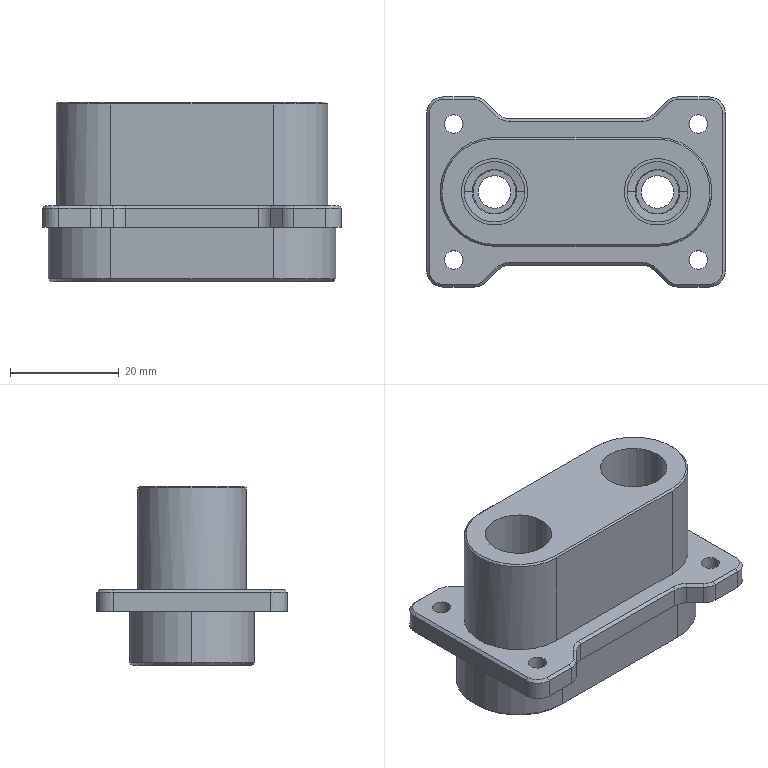NC program | NX | posted with a generic post | part box 55 x 35 x 33 mm
Whole program:
N10 G17 G21 G94 G90
(PLANAR_MILL , TOOL : D50面刀)
N12 T01 M6
N14 G54
N16 G17 G0 G90 X59.5 Y0. S3500 M3
N18 G43 Z30. H1
N20 Z2.
N22 G94 G1 Z0. F800.
N24 X29.5
N26 X-29.5
N28 X-59.5
N30 Z2.
N32 G0 Z30.
N34 M5
(ADAPTIVE_MILLING , TOOL : D6开粗)
N36 T02 M6
N38 G54
N40 G17 G0 G90 X-37.082 Y-1.951 S5500 M3
N42 G43 Z30. H2
N44 Z-6.85
N46 G94 G1 X-36.933 Y-1.933 Z-7.787 F2500.
N48 X-36.784 Y-1.915 Z-8.158
N50 X-36.635 Y-1.896 Z-8.43
N52 X-36.486 Y-1.878 Z-8.65
N54 X-36.337 Y-1.859 Z-8.834
N56 X-36.188 Y-1.841 Z-8.992
N58 X-36.04 Y-1.823 Z-9.13
N60 X-35.891 Y-1.804 Z-9.25
N62 X-35.742 Y-1.786 Z-9.355
N64 X-35.593 Y-1.767 Z-9.448
N66 X-35.444 Y-1.749 Z-9.529
N68 X-35.295 Y-1.731 Z-9.6
N70 X-35.146 Y-1.712 Z-9.66
N72 X-34.997 Y-1.694 Z-9.712
N74 X-34.849 Y-1.675 Z-9.755
N76 X-34.7 Y-1.657 Z-9.789
N78 X-34.551 Y-1.639 Z-9.816
N80 X-34.402 Y-1.62 Z-9.835
N82 X-34.253 Y-1.602 Z-9.846
N84 X-34.104 Y-1.583 Z-9.85
N86 X-33.036 Y-1.451
N88 G3 X-32.602 Y-1.181 R0.61
N90 X-32.052 Y0.418 R3.749
N92 X-31.757 Y5.239 R34.791
N94 G1 X-31.719 Y18.308
N96 G2 X-30.257 Y20.605 R3.404
N98 X-27.007 Y21.854 R7.591
N100 X-21.623 Y22.205 R36.427
N102 G1 X-15.224 Y22.23
N104 X27.708 Y22.226
N106 G2 X30.104 Y20.755 R3.359
N108 X31.371 Y17.403 R7.706
N110 X31.707 Y11.819 R39.238
N112 G1 X31.729 Y4.819
N114 X31.727 Y-18.149
N116 G2 X30.405 Y-20.517 R3.217
N118 X27.196 Y-21.824 R7.156
N120 X22.015 Y-22.193 R33.325
N122 G1 X15.015 Y-22.223
N124 X-27.647 Y-22.228
N126 G2 X-30.017 Y-20.909 R3.219
N128 X-31.327 Y-17.701 R7.175
N130 X-31.694 Y-12.72 R32.061
N132 X-31.711 Y-3.192 R449.115
N134 X-31.242 Y0.643 R185.492
N136 G3 X-30.94 Y8.619 R86.106
N138 G1 X-30.917 Y16.308
N140 G2 X-28.825 Y19.681 R4.499
N142 X-24.992 Y21.042 R9.424
N144 X-19.008 Y21.406 R44.006
N146 G1 X-12.408 Y21.43
N148 X25.608 Y21.427
N150 G2 X29.121 Y19.407 R4.476
N152 X30.525 Y15.588 R9.179
N154 X30.902 Y9.705 R41.842
N156 G1 X30.929 Y2.605
N158 X30.926 Y-16.168
N160 G2 X28.878 Y-19.655 R4.431
N162 X25.248 Y-20.997 R9.046
N164 X19.667 Y-21.389 R38.056
N166 G1 X13.067 Y-21.423
N168 X-25.667 Y-21.426
N170 G2 X-29.158 Y-19.377 R4.444
N172 X-30.519 Y-15.65 R9.202
N174 X-30.9 Y-9.867 R40.724
N176 X-30.878 Y-3.868 R96.242
N178 G1 X-30.404 Y1.28
N180 G3 X-30.135 Y10.714 R133.466
N182 G2 X-30.095 Y14.907 R80.862
N184 X-27.424 Y18.917 R5.279
N186 X-23.263 Y20.254 R11.082
N188 X-16.577 Y20.611 R53.243
N190 G1 X-9.977 Y20.629
N192 X23.823 Y20.627
N194 G2 X28.316 Y18.084 R5.223
N196 X29.708 Y14.049 R10.439
N198 X30.103 Y7.666 R46.614
N200 G1 X30.129 Y3.266
N202 X30.128 Y-14.268
N204 G2 X27.533 Y-18.852 R5.225
N206 X23.385 Y-20.231 R10.759
N208 X17.301 Y-20.596 R47.863
N210 G1 X10.701 Y-20.623
N212 X-23.768 Y-20.628
N214 G2 X-28.404 Y-17.959 R5.26
N216 X-29.734 Y-13.897 R10.825
N218 X-30.098 Y-8.013 R46.197
N220 X-29.753 Y-0.507 R61.506
N222 G3 X-29.338 Y10.918 R136.638
N224 G2 X-29.245 Y13.909 R23.846
N226 X-26.349 Y18.035 R5.781
N228 X-22.095 Y19.413 R11.597
N230 X-15.512 Y19.803 R50.356
N232 G1 X-8.912 Y19.829
N234 X22.188 Y19.827
N236 G2 X26.329 Y18.348 R5.861
N238 X28.494 Y14.571 R8.022
N240 X29.2 Y9.531 R22.93
N242 X29.322 Y2.969 R160.009
N244 G1 X29.541 Y1.782
N246 X29.65 Y0.018
N248 G3 X29.383 Y-4.527 R166.198
N250 X29.319 Y-13.068 R660.599
N252 G2 X26.406 Y-18.003 R5.745
N254 X22.144 Y-19.401 R11.531
N256 X15.56 Y-19.796 R50.199
N258 G1 X8.56 Y-19.823
N260 X-22.267 Y-19.826
N262 G2 X-27.607 Y-16.734 R5.839
N264 X-28.933 Y-12.461 R11.993
N266 X-29.178 Y-3.571 R47.724
N268 G1 X-29.398 Y-2.708
N270 X-29.624 Y-0.88
N272 X-29.618 Y0.964
N274 X-29.381 Y2.792
N276 G3 X-28.648 Y7.519 R17.936
N278 G1 X-28.51 Y12.137
N280 G2 X-25.151 Y17.278 R6.243
N282 X-20.671 Y18.631 R12.837
N284 X-13.785 Y19.006 R56.828
N286 G1 X-7.186 Y19.029
N288 X20.614 Y19.028
N290 G2 X23.929 Y18.419 R7.485
N292 X27.126 Y14.947 R6.784
N294 X28.247 Y10.198 R15.536
N296 X28.489 Y5.706 R68.839
N298 X29.221 Y3.52 R19.948
N300 G1 X29.541 Y1.782
N302 X29.65 Y0.018
N304 X29.545 Y-1.75
N306 X29.228 Y-3.491
N308 G3 X28.662 Y-6.813 R11.878
N310 X28.515 Y-11.988 R178.125
N312 G2 X25.189 Y-17.254 R6.207
N314 X20.613 Y-18.633 R12.848
N316 X13.527 Y-19.003 R59.413
N318 G1 X6.827 Y-19.023
N320 X-20.767 Y-19.026
N322 G2 X-24.245 Y-18.265 R7.08
N324 X-27.186 Y-14.821 R6.918
N326 X-28.262 Y-10.058 R16.145
N328 X-28.424 Y-5.863 R43.057
N330 G3 X-28.944 Y-4.494 R26.651
N332 G1 X-29.19 Y-3.525
N334 G3 X-30.311 Y-3.412 R0.6
N336 X-30.381 Y-3.799 Z-9.816 R0.993
N338 G1 X-30.431 Y-4.572 Z-9.75
N340 X-30.508 Y-5.808 F15000.
N342 X-30.457 Y-6.903
N344 X-30.379 Y-7.995
N346 X-30.249 Y-9.083
N348 X-30.03 Y-10.643
N350 X-29.795 Y-12.2
N352 G3 X-28.906 Y-15.512 R18.855
N354 X-27.408 Y-17.991 R8.282
N356 X-25.771 Y-19.435 R9.961
N358 X-22.736 Y-20.597 R6.897
N360 X-20.187 Y-20.803 R24.199
N362 G1 X-11.768 Y-21.022
N364 G3 X7.264 Y-20.986 R342.154
N366 G1 X17.513 Y-20.682
N368 G3 X21.869 Y-20.217 R28.725
N370 G1 X23.306 Y-19.944
N372 G3 X26.593 Y-18.44 R8.595
N374 G1 X27.535 Y-17.671
N376 X28.462 Y-16.883
N378 G3 X29.175 Y-15.926 R3.574
N380 X29.882 Y-14.324 R14.731
N382 X30.131 Y-13.189 R5.303
N384 G1 X30.884 Y-6.024
N386 G3 X30.839 Y-5.725 R0.642
N388 G1 X30.401 Y-4.7
N390 X30.255 Y-4.352 Z-9.782 F2500.
N392 X30.096 Y-4.01 Z-9.814
N394 G3 X29.769 Y-3.764 Z-9.85 R0.623
N396 X29.02 Y-4.16 R0.6
N398 G2 X28.376 Y-5.971 R15.766
N400 G3 X27.867 Y-9.311 R14.098
N402 G2 X27.561 Y-12.173 R15.984
N404 X24.062 Y-16.49 R6.653
N406 X19.377 Y-17.835 R13.823
N408 X12.491 Y-18.199 R60.434
N410 G1 X5.891 Y-18.223
N412 X-19.209 Y-18.226
N414 G2 X-22.461 Y-17.781 R9.236
N416 X-26.01 Y-14.517 R6.661
N418 X-27.342 Y-9.827 R13.693
N420 X-27.535 Y-7.607 R122.141
N422 G1 X-27.571 Y-7.485
N424 X-28.269 Y-6.209
N426 X-28.452 Y-5.744
N428 G3 X-29.411 Y-5.517 R0.6
N430 X-29.618 Y-6.022 Z-9.802 R0.677
N432 G1 X-29.671 Y-6.629 Z-9.75
N434 X-29.732 Y-7.285 F15000.
N436 X-29.781 Y-7.942
N438 X-29.77 Y-8.027
N440 X-29.493 Y-9.416
N442 X-29.207 Y-10.802
N444 G3 X-28.089 Y-14.361 R23.376
N446 G1 X-27.829 Y-15.008
N448 X-27.557 Y-15.651
N450 G3 X-26.493 Y-17.163 R5.423
N452 X-24.494 Y-18.742 R8.627
N454 X-22.483 Y-19.584 R10.598
N456 X-20.874 Y-19.884 R9.996
N458 G1 X-20.056 Y-19.959
N460 X-19.235 Y-20.001
N462 X-13.012 Y-20.173
N464 G3 X1.628 Y-20.213 R296.226
N466 G1 X17.37 Y-19.867
N468 G3 X20.984 Y-19.414 R17.804
N470 X22.961 Y-18.887 R18.627
N472 X25.999 Y-17.326 R11.757
N474 X27.39 Y-16.258 R13.751
N476 X28.716 Y-14.362 R5.779
N478 X29.328 Y-12.337 R9.804
N480 X29.644 Y-10.168 R16.371
N482 G1 X29.816 Y-7.922
N484 Y-7.824
N486 X29.705 Y-6.553
N488 X29.672 Y-6.148 Z-9.785 F2500.
N490 X29.629 Y-5.744 Z-9.819
N492 G3 X29.448 Y-5.44 Z-9.85 R0.629
N494 X28.498 Y-5.638 R0.6
N496 X27.66 Y-7.509 R46.066
N498 X27.088 Y-10.236 R19.372
N500 G2 X22.823 Y-15.81 R7.311
N502 X18.093 Y-17.054 R15.354
N504 X10.905 Y-17.402 R67.473
N506 G1 X4.005 Y-17.423
N508 X-17.895 Y-17.425
N510 G2 X-21.256 Y-17.029 R10.737
N512 X-25.118 Y-13.651 R6.841
N514 X-26.465 Y-9.19 R13.593
N516 G1 X-26.54 Y-8.992
N518 X-27.384 Y-7.826
N520 X-27.576 Y-7.475
N522 G3 X-28.681 Y-7.603 R0.6
N524 X-28.669 Y-7.991 Z-9.816 R0.761
N526 G1 X-28.515 Y-8.754 Z-9.75
N528 G3 X-27.755 Y-11.932 R30.929 F15000.
N530 X-26.724 Y-14.509 R21.421
N532 X-25.414 Y-16.522 R10.735
N534 X-23.567 Y-17.923 R6.211
N536 X-19.903 Y-19.057 R9.881
N538 G1 X-19.467 Y-19.094
N540 X-19.031 Y-19.119
N542 X-10.979 Y-19.366
N544 G3 X7.317 Y-19.339 R284.305
N546 G1 X16.101 Y-19.043
N548 G3 X21.033 Y-18.331 R22.731
N550 X22.859 Y-17.676 R13.177
N552 X24.83 Y-16.717 R20.702
N554 X26.254 Y-15.589 R6.643
N556 X27.806 Y-13.574 R9.266
N558 X28.875 Y-10.891 R8.615
N560 G1 X29.244 Y-9.166
N562 X29.254 Y-9.069
N564 X29.253 Y-8.971
N566 X29.113 Y-7.778
N568 X29.071 Y-7.399 Z-9.783 F2500.
N570 X29.015 Y-7.023 Z-9.815
N572 G3 X28.778 Y-6.698 Z-9.85 R0.623
N574 X27.926 Y-6.883 R0.6
N576 X26.466 Y-9.968 R11.481
N578 G2 X21.242 Y-15.291 R8.422
N580 X15.967 Y-16.364 R19.661
N582 X7.373 Y-16.617 R110.307
N584 G1 X2.973 Y-16.623
N586 X-16.667 Y-16.625
N588 G2 X-19.943 Y-16.312 R12.654
N590 X-24.295 Y-12.691 R6.987
N592 X-25.162 Y-10.574 R15.381
N594 G1 X-25.223 Y-10.473
N596 X-26.304 Y-9.319
N598 X-26.597 Y-8.914
N600 G3 X-27.583 Y-8.934 R0.6
N602 X-27.656 Y-9.474 Z-9.802 R0.677
N604 G1 X-27.557 Y-10.076 Z-9.75
N606 X-27.345 Y-11.317 F15000.
N608 X-27.279 Y-11.461
N610 X-25.841 Y-13.727
N612 G3 X-24.335 Y-15.636 R16.325
N614 G1 X-23.636 Y-16.384
N616 G3 X-21.395 Y-17.697 R5.625
N618 X-18.365 Y-18.301 R11.912
N620 G1 X-17.545 Y-18.353
N622 X-16.723 Y-18.378
N624 X6.345 Y-18.637
N626 G3 X15.109 Y-18.236 R77.021
N628 G1 X16.644 Y-18.079
N630 X18.177 Y-17.911
N632 G3 X21.222 Y-17.221 R17.457
N634 G1 X21.917 Y-16.997
N636 X22.601 Y-16.742
N638 G3 X25.567 Y-14.668 R9.098
N640 X27.612 Y-11.993 R12.284
N642 G1 X28.572 Y-10.279
N644 G3 X28.641 Y-9.887 R0.61
N646 G1 X28.467 Y-8.851
N648 X28.408 Y-8.477 Z-9.782 F2500.
N650 X28.334 Y-8.107 Z-9.815
N652 G3 X28.076 Y-7.791 Z-9.85 R0.623
N654 X27.254 Y-7.996 R0.6
N656 G2 X26.385 Y-9.18 R9.511
N658 X24.541 Y-11.751 R24.024
N660 X19.344 Y-14.834 R10.566
N662 X13.314 Y-15.675 R27.91
N664 X3.916 Y-15.82 R212.096
N666 G1 X-0.084 Y-15.823
N668 X-15.384 Y-15.824
N670 G2 X-18.862 Y-15.529 R14.424
N672 X-23.284 Y-12.115 R7.13
N674 G3 X-23.625 Y-11.842 R1.3
N676 G1 X-25.044 Y-10.665
N678 X-25.249 Y-10.446
N680 G3 X-26.285 Y-10.805 R0.6
N682 X-26.179 Y-11.218 Z-9.813 R0.733
N684 G1 X-25.86 Y-11.885 Z-9.75
N686 X-25.366 Y-12.917 F15000.
N688 X-25.313 Y-13.003
N690 X-25.249 Y-13.082
N692 X-24.102 Y-14.234
N694 X-22.944 Y-15.376
N696 G3 X-20.775 Y-16.708 R6.83
N698 X-17.779 Y-17.453 R10.843
N700 G1 X-16.961 Y-17.529
N702 X-16.14 Y-17.574
N704 G3 X-9.552 Y-17.689 R147.707
N706 G1 X12.417 Y-17.532
N708 G3 X17.501 Y-17.046 R29.086
N710 G1 X19.058 Y-16.749
N712 G3 X23.514 Y-14.935 R13.903
N714 X26.047 Y-12.824 R13.025
N716 G1 X27.067 Y-11.726
N718 G3 X27.223 Y-11.395 R0.614
N720 G1 X27.362 Y-10.323
N722 X27.415 Y-9.929 Z-9.784 F2500.
N724 X27.457 Y-9.533 Z-9.818
N726 G3 X27.334 Y-9.185 Z-9.85 R0.627
N728 X26.385 Y-9.18 R0.6
N730 G1 X25.972 Y-9.708
N732 X24.72 Y-10.961
N734 X23.327 Y-12.053
N736 X21.812 Y-12.97
N738 X20.198 Y-13.697
N740 X18.508 Y-14.224
N742 G2 X13.38 Y-14.836 R31.101
N744 X2.782 Y-15.02 R209.061
N746 G1 X-1.618 Y-15.023
N748 X-14.318
N750 G2 X-17.896 Y-14.723 R15.402
N752 X-20.276 Y-13.659 R7.237
N754 X-22.07 Y-12.831 R93.694
N756 G1 X-23.42 Y-11.972
N758 G3 X-24.303 Y-12.693 R0.6
N760 G1 X-24.209 Y-12.854 Z-9.834
N762 X-24.09 Y-12.997 Z-9.818
N764 X-23.574 Y-13.606 Z-9.75
N766 X-22.871 Y-14.428 F15000.
N768 X-22.738 Y-14.519
N770 X-21.43 Y-15.177
N772 X-20.115 Y-15.822
N774 G3 X-17.533 Y-16.555 R9.687
N776 G1 X-16.882 Y-16.63
N778 X-16.228 Y-16.672
N780 G3 X-10.74 Y-16.788 R153.009
N782 G1 X15.448 Y-16.826
N784 G3 X15.824 Y-16.695 R0.61
N786 G1 X16.658 Y-16.027
N788 X16.959 Y-15.789 Z-9.783 F2500.
N790 X17.251 Y-15.541 Z-9.816
N792 G3 X17.402 Y-15.173 Z-9.85 R0.624
N794 X16.766 Y-14.543 R0.6
N796 G1 X15. Y-14.65
N798 X-15.
N800 X-16.84 Y-14.534
N802 X-18.651 Y-14.188
N804 X-20.362 Y-13.63
N806 G3 X-20.917 Y-13.728 R0.602
N808 G1 X-21.066 Y-13.887 Z-9.831
N810 X-21.197 Y-14.062 Z-9.813
N812 X-21.643 Y-14.646 Z-9.75
N814 X-21.857 Y-14.915 F15000.
N816 G2 X-22.645 Y-14.949 R0.6
N818 G1 X-25.791 Y-12.433
N820 G2 X-28.173 Y-9.876 R12.602
N822 X-30.188 Y-6.239 R19.345
N824 G1 X-30.521 Y-5.435
N826 X-30.824 Y-4.619
N828 G2 X-31.386 Y-0.872 R11.284
N830 G1 X-31.312 Y2.829
N832 G2 X-30.845 Y3.402 R0.601
N834 G1 X-30.75 Y3.423
N836 X-29.608 Y3.683 Z-9.85 F2500.
N838 G3 X-29.226 Y3.836 R0.804
N840 X-29.029 Y4.147 R0.614
N842 G2 X-28.434 Y5.783 R10.409
N844 G3 X-27.877 Y9.353 R14.406
N846 G2 X-27.529 Y12.313 R15.141
N848 X-24.043 Y16.503 R6.657
N850 X-19.552 Y17.818 R13.573
N852 X-13.068 Y18.197 R54.895
N854 G1 X-5.268 Y18.228
N856 X19.232 Y18.227
N858 G2 X22.575 Y17.734 R8.942
N860 X26.146 Y14.24 R6.83
N862 X27.384 Y9.522 R14.721
N864 G3 X27.587 Y7.475 R67.601
N866 G2 X28.542 Y5.543 R14.098
N868 G3 X29.455 Y5.314 R0.6
N870 X29.697 Y5.845 Z-9.799 R0.676
N872 G1 X29.751 Y6.41 Z-9.75
N874 X29.818 Y7.074 F15000.
N876 X29.871 Y7.739
N878 X29.86 Y7.826
N880 X29.374 Y10.217
N882 G3 X28.501 Y13.131 R22.991
N884 G1 X28.133 Y14.123
N886 X27.753 Y15.11
N888 G3 X26.324 Y17.22 R6.753
N890 G1 X25.86 Y17.686
N892 X25.377 Y18.133
N894 G3 X23.372 Y19.302 R6.415
N896 X20.9 Y19.86 R8.371
N898 X16.514 Y20.063 R106.973
N900 G1 X7.363 Y20.286
N902 G3 X-10.203 Y20.133 R266.298
N904 G1 X-13.808 Y19.986
N906 X-17.413 Y19.825
N908 G3 X-21.138 Y19.341 R28.822
N910 G1 X-21.856 Y19.2
N912 X-22.573 Y19.049
N914 G3 X-24.585 Y18.236 R8.206
N916 X-26.437 Y17.065 R12.937
N918 X-28.161 Y15.197 R7.295
N920 X-29.073 Y13.233 R6.421
N922 X-29.832 Y10.032 R42.782
N924 G1 X-30.298 Y7.647
N926 G3 X-30.252 Y7.276 R0.613
N928 G1 X-29.809 Y6.335
N930 X-29.491 Y5.674 Z-9.813 F2500.
N932 G3 X-29.142 Y5.425 Z-9.85 R0.618
N934 X-28.434 Y5.783 R0.6
N936 G2 X-27.815 Y7.071 R10.863
N938 G3 X-27.172 Y9.779 R11.857
N940 G2 X-25.697 Y13.557 R8.087
N942 X-21.694 Y16.278 R8.352
N944 X-16.393 Y17.225 R21.072
N946 X-7.297 Y17.426 R140.115
N948 G1 X-3.997 Y17.428
N950 X17.903 Y17.427
N952 G2 X21.263 Y17.023 R10.572
N954 X25.166 Y13.553 R6.883
N956 X26.483 Y9.168 R13.994
N958 G1 X26.572 Y8.941
N960 G2 X27.62 Y7.39 R9.642
N962 G3 X28.705 Y7.517 R0.6
N964 X28.7 Y7.931 Z-9.814 R0.755
N966 G1 X28.554 Y8.668 Z-9.75
N968 X28.303 Y9.936 F15000.
N970 X28.064 Y10.895
N972 X27.799 Y11.846
N974 G3 X26.768 Y14.424 R21.421
N976 X25.458 Y16.437 R10.735
N978 X24.246 Y17.48 R6.309
N980 X22.323 Y18.514 R10.726
N982 X19.989 Y19.062 R9.324
N984 G1 X19.553 Y19.098
N986 X19.116 Y19.121
N988 X6.673 Y19.455
N990 G3 X-10.158 Y19.302 R234.294
N992 G1 X-16.743 Y19.005
N994 G3 X-23.336 Y17.573 R19.764
N996 X-24.722 Y16.931 R14.208
N998 X-26.46 Y15.528 R6.763
N1000 X-28.683 Y11.406 R9.074
N1002 G1 X-29.211 Y9.182
N1004 X-29.224 Y9.08
N1006 X-29.223 Y8.977
N1008 X-29.089 Y7.788
N1010 X-29.049 Y7.405 Z-9.783 F2500.
N1012 X-28.994 Y7.024 Z-9.816
N1014 G3 X-28.767 Y6.702 Z-9.85 R0.624
N1016 X-27.893 Y6.899 R0.6
N1018 X-26.421 Y10.109 R14.592
N1020 G2 X-21.39 Y15.24 R8.377
N1022 X-16.125 Y16.357 R18.963
N1024 X-7.431 Y16.622 R106.756
N1026 G1 X-3.031 Y16.628
N1028 X16.669 Y16.627
N1030 G2 X20.136 Y16.254 R11.999
N1032 X24.24 Y12.793 R6.971
N1034 X25.192 Y10.519 R15.847
N1036 G3 X25.96 Y9.722 R6.483
N1038 G1 X26.577 Y8.935
N1040 G3 X27.528 Y8.943 R0.6
N1042 X27.623 Y9.513 Z-9.799 R0.68
N1044 G1 X27.533 Y10.08 Z-9.75
N1046 X27.434 Y10.708 F15000.
N1048 X27.326 Y11.335
N1050 X27.259 Y11.481
N1052 X25.821 Y13.748
N1054 G3 X24.315 Y15.657 R16.325
N1056 G1 X23.616 Y16.404
N1058 G3 X21.375 Y17.717 R5.625
N1060 X18.523 Y18.27 R10.536
N1062 X15.602 Y18.402 R44.81
N1064 G1 X-6.368 Y18.653
N1066 G3 X-15.133 Y18.253 R77.072
N1068 G1 X-16.832 Y18.081
N1070 X-18.529 Y17.895
N1072 G3 X-23.551 Y16.156 R13.46
N1074 G1 X-24.158 Y15.798
N1076 X-24.76 Y15.431
N1078 G3 X-26.116 Y14.172 R5.813
N1080 X-27.352 Y12.366 R18.057
N1082 G1 X-28.661 Y10.174
N1084 G3 X-28.735 Y9.751 R0.608
N1086 G1 X-28.541 Y8.762
N1088 X-28.393 Y8.045 Z-9.813 F2500.
N1090 G3 X-28.114 Y7.718 Z-9.85 R0.618
N1092 X-27.343 Y7.891 R0.6
N1094 X-25.165 Y10.993 R85.559
N1096 G2 X-19.721 Y14.729 R10.251
N1098 X-13.907 Y15.647 R25.164
N1100 X-4.51 Y15.825 R172.453
N1102 G1 X-0.11 Y15.827
N1104 X15.29
N1106 G2 X18.868 Y15.527 R14.787
N1108 X23.237 Y12.193 R7.082
N1110 G1 X23.364 Y12.023
N1112 X24.709 Y10.971
N1114 X25.275 Y10.405
N1116 G3 X26.298 Y10.804 R0.6
N1118 X26.194 Y11.187 Z-9.816 R0.752
N1120 G1 X25.864 Y11.882 Z-9.75
N1122 X25.393 Y12.875 F15000.
N1124 X25.339 Y12.962
N1126 X25.275 Y13.042
N1128 X24.113 Y14.209
N1130 X22.94 Y15.365
N1132 G3 X21.33 Y16.49 R7.159
N1134 X17.977 Y17.406 R10.026
N1136 X15.063 Y17.623 R35.441
N1138 X6.645 Y17.751 R171.588
N1140 G1 X-13.494 Y17.514
N1142 G3 X-20.217 Y16.441 R23.767
N1144 X-22.702 Y15.472 R26.084
N1146 X-24.568 Y14.255 R8.291
N1148 X-25.837 Y13.071 R16.104
N1150 G1 X-26.943 Y11.918
N1152 G3 X-27.106 Y11.567 R0.611
N1154 G1 X-27.222 Y10.503
N1156 X-27.266 Y10.125 Z-9.783 F2500.
N1158 X-27.296 Y9.746 Z-9.815
N1160 G3 X-27.137 Y9.376 Z-9.85 R0.623
N1162 X-26.261 Y9.371 R0.6
N1164 G1 X-25.002 Y10.704
N1166 X-23.586 Y11.87
N1168 X-22.036 Y12.85
N1170 X-20.375 Y13.628
N1172 X-18.631 Y14.193
N1174 G2 X-13.443 Y14.836 R30.112
N1176 X-2.046 Y15.025 R218.585
N1178 G1 X13.608 Y15.027
N1180 G2 X17.398 Y14.829 R22.082
N1182 X20.213 Y13.69 R7.067
N1184 G1 X21.804 Y12.974
N1186 X23.396 Y11.999
N1188 G3 X24.319 Y12.702 R0.6
N1190 G1 X24.225 Y12.856 Z-9.835
N1192 X24.108 Y12.994 Z-9.819
N1194 X23.58 Y13.607 Z-9.75
N1196 X22.845 Y14.456 F15000.
N1198 X22.713 Y14.545
N1200 X21.406 Y15.203
N1202 X20.092 Y15.848
N1204 G3 X17.07 Y16.631 R9.762
N1206 G1 X16.633 Y16.664
N1208 X16.196 Y16.684
N1210 G3 X7.413 Y16.796 R426.412
N1212 G1 X-15.511 Y16.818
N1214 G3 X-15.887 Y16.687 R0.61
N1216 G1 X-16.72 Y16.02
N1218 X-17.022 Y15.782 Z-9.783 F2500.
N1220 X-17.315 Y15.533 Z-9.816
N1222 G3 X-17.466 Y15.168 Z-9.85 R0.624
N1224 X-16.829 Y14.535 R0.6
N1226 G1 X-15. Y14.65
N1228 X15.
N1230 X16.765 Y14.543
N1232 X18.504 Y14.225
N1234 X20.283 Y13.658
N1236 G3 X21.061 Y13.917 R0.606
N1238 G1 X21.505 Y14.715
N1240 X21.577 Y14.846 Z-9.846
N1242 X21.65 Y14.977 Z-9.835
N1244 X21.723 Y15.108 Z-9.816
N1246 X21.796 Y15.239 Z-9.789
N1248 X21.869 Y15.37 Z-9.755
N1250 X21.942 Y15.501 Z-9.712
N1252 X22.014 Y15.633 Z-9.66
N1254 X22.087 Y15.764 Z-9.6
N1256 X22.16 Y15.895 Z-9.529
N1258 X22.233 Y16.026 Z-9.448
N1260 X22.306 Y16.157 Z-9.355
N1262 X22.379 Y16.288 Z-9.25
N1264 X22.451 Y16.419 Z-9.13
N1266 X22.524 Y16.55 Z-8.992
N1268 X22.597 Y16.682 Z-8.834
N1270 X22.67 Y16.813 Z-8.65
N1272 X22.743 Y16.944 Z-8.43
N1274 X22.816 Y17.075 Z-8.158
N1276 X22.888 Y17.206 Z-7.787
N1278 X22.961 Y17.337 Z-6.85
N1280 G0 Z30.
N1282 X-37.058 Y-0.827
N1284 Z-13.
N1286 G1 X-36.909 Y-0.808 Z-13.937
N1288 X-36.76 Y-0.79 Z-14.308
N1290 X-36.611 Y-0.771 Z-14.58
N1292 X-36.462 Y-0.752 Z-14.8
N1294 X-36.313 Y-0.733 Z-14.984
N1296 X-36.165 Y-0.715 Z-15.142
N1298 X-36.016 Y-0.696 Z-15.28
N1300 X-35.867 Y-0.677 Z-15.4
N1302 X-35.718 Y-0.659 Z-15.505
N1304 X-35.569 Y-0.64 Z-15.598
N1306 X-35.42 Y-0.621 Z-15.679
N1308 X-35.272 Y-0.602 Z-15.75
N1310 X-35.123 Y-0.584 Z-15.81
N1312 X-34.974 Y-0.565 Z-15.862
N1314 X-34.825 Y-0.546 Z-15.905
N1316 X-34.676 Y-0.528 Z-15.939
N1318 X-34.527 Y-0.509 Z-15.966
N1320 X-34.379 Y-0.49 Z-15.985
N1322 X-34.23 Y-0.471 Z-15.996
N1324 X-34.081 Y-0.453 Z-16.
N1326 X-33.009 Y-0.318
N1328 G3 X-32.579 Y-0.05 R0.61
N1330 X-32.039 Y1.473 R3.615
N1332 X-31.73 Y6.271 R32.681
N1334 G1 X-31.694 Y18.238
N1336 G2 X-30.204 Y20.621 R3.354
N1338 X-26.856 Y21.853 R7.741
N1340 X-21.471 Y22.177 R39.254
N1342 G1 X-15.171 Y22.2
N1344 X27.638 Y22.199
N1346 G2 X30. Y20.863 R3.23
N1348 X31.302 Y17.652 R7.204
N1350 X31.666 Y12.57 R32.696
N1352 G1 X31.699 Y3.571
N1354 X31.698 Y-18.138
N1356 G2 X30.364 Y-20.5 R3.229
N1358 X27.149 Y-21.802 R7.222
N1360 X22.067 Y-22.168 R32.916
N1362 G1 X15.068 Y-22.2
N1364 X-27.62 Y-22.198
N1366 G2 X-29.989 Y-20.877 R3.22
N1368 X-31.298 Y-17.668 R7.182
N1370 X-31.665 Y-12.587 R32.431
N1372 X-31.682 Y-2.063 R581.846
N1374 X-31.223 Y1.679 R142.019
N1376 G3 X-30.912 Y9.85 R85.166
N1378 G1 X-30.885 Y16.338
N1380 G2 X-28.767 Y19.685 R4.505
N1382 X-24.925 Y21.023 R9.496
N1384 X-19.04 Y21.374 R44.192
N1386 G1 X-11.871 Y21.4
N1388 X25.638 Y21.396
N1390 G2 X29.184 Y19.265 R4.495
N1392 X30.381 Y16.195 R8.731
N1394 X30.673 Y14.507 R6.271
N1396 X30.892 Y6.912 R92.476
N1398 G1 X30.899 Y0.912
N1400 X30.896 Y-16.138
N1402 G2 X28.847 Y-19.629 R4.443
N1404 X25.1 Y-20.994 R9.188
N1406 X19.617 Y-21.365 R39.088
N1408 G1 X11.872 Y-21.4
N1410 X-25.638 Y-21.396
N1412 G2 X-29.184 Y-19.265 R4.494
N1414 X-30.381 Y-16.197 R8.735
N1416 X-30.673 Y-14.507 R6.27
N1418 X-30.892 Y-6.912 R92.47
N1420 G1 X-30.897 Y-4.512
N1422 Y11.688
N1424 G2 X-30.659 Y12.328 R10.379
N1426 G1 X-30.65 Y14.501
N1428 X-30.531 Y15.701
N1430 X-30.181 Y16.855
N1432 X-29.613 Y17.918
N1434 X-28.848 Y18.85
N1436 X-27.915 Y19.614
N1438 X-26.852 Y20.182
N1440 X-25.698 Y20.532
N1442 X-24.499 Y20.65
N1444 G2 X-14.855 Y20.605 R707.909
N1446 G1 X-11.262 Y20.599
N1448 X18.227
N1450 X18.743 Y20.65
N1452 X24.501
N1454 X25.701 Y20.531
N1456 X26.855 Y20.181
N1458 X27.918 Y19.613
N1460 X28.85 Y18.848
N1462 X29.614 Y17.915
N1464 X30.182 Y16.852
N1466 X30.532 Y15.698
N1468 X30.65 Y14.499
N1470 Y-14.501
N1472 X30.531 Y-15.701
N1474 X30.181 Y-16.855
N1476 X29.613 Y-17.918
N1478 X28.848 Y-18.85
N1480 X27.915 Y-19.614
N1482 X26.852 Y-20.182
N1484 X25.698 Y-20.532
N1486 X24.499 Y-20.65
N1488 G2 X14.856 Y-20.605 R706.013
N1490 G1 X-18.228 Y-20.599
N1492 X-18.743 Y-20.65
N1494 X-24.501
N1496 X-25.701 Y-20.531
N1498 X-26.855 Y-20.181
N1500 X-27.918 Y-19.613
N1502 X-28.85 Y-18.848
N1504 X-29.614 Y-17.915
N1506 X-30.182 Y-16.852
N1508 X-30.385 Y-16.182
N1510 G3 X-31.363 Y-15.912 R0.6
N1512 X-31.57 Y-16.389 Z-15.955 R0.695
N1514 G1 X-31.657 Y-17.022 Z-15.9
N1516 X-31.736 Y-17.579 F15000.
N1518 X-31.804 Y-18.137
N1520 G3 X-31.704 Y-18.465 R0.619
N1522 G1 X-31.467 Y-18.819
N1524 X-31.201 Y-19.153
N1526 X-30.352 Y-19.975
N1528 X-29.485 Y-20.779
N1530 G3 X-27.164 Y-21.954 R5.897
N1532 X-24.654 Y-22.344 R10.078
N1534 G1 X-21.36 Y-22.409
N1536 X-18.066 Y-22.438
N1538 X16.949 Y-22.51
N1540 X17.087 Y-22.477
N1542 X18.178 Y-22.073
N1544 X18.584 Y-21.927 Z-15.937 F2500.
N1546 X18.984 Y-21.766 Z-15.974
N1548 X19.105 Y-21.671 Z-15.987
N1550 X19.201 Y-21.55 Z-16.
N1552 G3 X18.742 Y-20.65 R0.6
N1554 G1 X17.541 Y-20.531
N1556 G3 X13.932 Y-19.915 R12.382
N1558 X5.262 Y-19.799 R188.82
N1560 G1 X-15.637 Y-19.812
N1562 G3 X-16.391 Y-20.182 R4.123
N1564 G1 X-17.544 Y-20.532
N1566 X-18.241 Y-20.601
N1568 G3 X-18.211 Y-21.916 R0.66
N1570 G1 X-17.039 Y-21.906 Z-15.9
N1572 X15.913 Y-21.567 F15000.
N1574 X16.253 Y-21.565 Z-15.929 F2500.
N1576 X16.593 Y-21.553 Z-15.958
N1578 G3 X17.007 Y-21.31 Z-16. R0.678
N1580 X16.68 Y-20.27 R0.66
N1582 G2 X15.771 Y-19.851 R3.601
N1584 G3 X12.753 Y-19.204 R9.755
N1586 X4.96 Y-19.001 R103.443
N1588 G1 X-13.636 Y-18.999
N1590 G3 X-14.622 Y-19.074 R3.484
N1592 X-15.327 Y-19.614 R4.252
N1594 G1 X-15.768 Y-19.85
N1596 G3 X-16.038 Y-20.746 R0.66
N1598 X-15.4 Y-21.092 Z-15.935 R0.675
N1600 G1 X-14.995 Z-15.9
N1602 X14.977 Y-21.093 F15000.
N1604 X15.557 Y-21.086 Z-15.95 F2500.
N1606 G3 X16.03 Y-20.765 Z-16. R0.67
N1608 X15.771 Y-19.851 R0.66
N1610 G2 X14.877 Y-19.296 R6.799
N1612 G3 X12.142 Y-18.533 R8.041
N1614 X6.237 Y-18.224 R52.48
N1616 G1 X1.862 Y-18.199
N1618 X-12.227 Y-18.2
N1620 G3 X-13.75 Y-18.307 R8.119
N1622 G1 X-13.97 Y-18.425
N1624 G2 X-14.781 Y-19.166 R8.123
N1626 G3 X-14.95 Y-19.977 R0.66
N1628 X-14.313 Y-20.337 Z-15.934 R0.674
N1630 G1 X-13.916 Y-20.342 Z-15.9
N1632 X14.27 Y-20.651 F15000.
N1634 X14.844 Y-20.649 Z-15.949 F2500.
N1636 G3 X15.323 Y-20.327 Z-16. R0.67
N1638 X15.17 Y-19.486 R0.66
N1640 X13.796 Y-18.496 R6.579
N1642 X10.499 Y-17.7 R10.661
N1644 X3.545 Y-17.416 R72.377
N1646 G1 X-4.038 Y-17.4
N1648 G3 X-12.042 Y-17.428 R361.233
N1650 X-13.088 Y-17.59 R3.509
N1652 G1 X-13.213 Y-17.668
N1654 X-13.991 Y-18.445
N1656 G3 X-14.104 Y-19.227 R0.661
N1658 X-13.428 Y-19.574 Z-15.932 R0.701
N1660 G1 X-13.06 Y-19.579 Z-15.9
N1662 X13.441 Y-19.968 F15000.
N1664 X14.016 Y-19.969 Z-15.949 F2500.
N1666 G3 X14.496 Y-19.65 Z-16. R0.67
N1668 X14.393 Y-18.848 R0.66
N1670 X12.038 Y-17.412 R4.599
N1672 X7.433 Y-16.755 R20.724
N1674 G1 X4.544 Y-16.65
N1676 X-11.153 Y-16.658
N1678 G3 X-12.299 Y-16.814 R4.651
N1680 G1 X-12.451 Y-16.906
N1682 X-13.229 Y-17.683
N1684 G3 X-13.082 Y-18.727 R0.66
N1686 X-12.384 Y-18.702 Z-15.938 R0.716
N1688 G1 X-11.985 Y-18.516 Z-15.9
N1690 X-11.133 Y-18.12 F15000.
N1692 X-10.594 Y-17.862 Z-15.951 F2500.
N1694 G3 X-10.301 Y-17.39 Z-16. R0.67
N1696 X-10.956 Y-16.65 R0.66
N1698 X-12.049 Y-16.67 R19.939
N1700 X-12.487 Y-16.942 R0.954
N1702 X-12.65 Y-17.491 R0.602
N1704 G1 X-12.597 Y-17.74
N1706 X-12.355 Y-18.886 Z-15.9
N1708 G2 X-12.337 Y-19.325 R0.836 F15000.
N1710 G1 X-12.397 Y-19.461
N1712 X-12.487 Y-19.579
N1714 X-13.489 Y-20.57
N1716 G2 X-17.104 Y-22.244 R6.788
N1718 X-19.287 Y-22.41 R17.093
N1720 G1 X-24.049 Y-22.461
N1722 G2 X-27.993 Y-21.681 R9.764
N1724 X-30.117 Y-20.191 R7.357
N1726 X-31.037 Y-19.113 R8.653
N1728 G1 X-31.85 Y-17.981
N1730 G2 X-31.775 Y-17.196 R0.6
N1732 G1 X-31.658 Y-17.084
N1734 X-30.807 Y-16.278 Z-16. F2500.
N1736 G3 X-30.542 Y-15.88 R0.735
N1738 G1 X-30.532 Y-15.698
N1740 X-30.65 Y-14.5
N1742 Y12.4
N1744 G3 X-30.923 Y12.903 R0.602
N1746 G1 X-31.13 Y13.038
N1748 X-32.112 Y13.677 Z-15.9
N1750 G2 X-32.442 Y13.978 R0.852 F15000.
N1752 G1 X-32.494 Y14.117
N1754 X-32.514 Y14.264
N1756 G2 X-32.435 Y15.354 R4.727
N1758 G1 X-32.245 Y16.221
N1760 X-32.046 Y17.086
N1762 G2 X-29.593 Y20.646 R6.531
N1764 X-25.53 Y22.314 R8.575
N1766 X-23.786 Y22.456 R14.259
N1768 G1 X-20.606 Y22.514
N1770 G2 X-20.1 Y22.253 R0.602
N1772 G1 X-20.012 Y22.125
N1774 X-19.35 Y21.159 Z-16. F2500.
N1776 X-19.235 Y20.99
N1778 X-19.112 Y20.827
N1780 G3 X-18.742 Y20.65 R0.609
N1782 G1 X-17.541 Y20.531
N1784 G3 X-13.931 Y19.915 R12.393
N1786 X-3.861 Y19.799 R222.961
N1788 G1 X15.62 Y19.81
N1790 G3 X16.391 Y20.182 R3.519
N1792 G1 X17.544 Y20.532
N1794 X18.241 Y20.601
N1796 G3 X18.211 Y21.916 R0.66
N1798 G1 X17.039 Y21.906 Z-15.9
N1800 X-15.913 Y21.567 F15000.
N1802 X-16.253 Y21.565 Z-15.929 F2500.
N1804 X-16.593 Y21.553 Z-15.958
N1806 G3 X-17.007 Y21.31 Z-16. R0.678
N1808 X-16.68 Y20.27 R0.66
N1810 G2 X-15.771 Y19.851 R3.601
N1812 G3 X-12.842 Y19.214 R9.403
N1814 X-6.85 Y19.01 R77.18
N1816 G1 X-2.461 Y18.999
N1818 X13.535 Y18.996
N1820 G3 X14.602 Y19.065 R4.492
N1822 X15.327 Y19.614 R3.662
N1824 G1 X15.768 Y19.85
N1826 G3 X16.038 Y20.746 R0.66
N1828 X15.4 Y21.092 Z-15.935 R0.675
N1830 G1 X14.995 Z-15.9
N1832 X-14.977 Y21.093 F15000.
N1834 X-15.557 Y21.086 Z-15.95 F2500.
N1836 G3 X-16.03 Y20.765 Z-16. R0.67
N1838 X-15.771 Y19.851 R0.66
N1840 G2 X-14.876 Y19.295 R6.78
N1842 G3 X-12.141 Y18.533 R8.074
N1844 X-6.236 Y18.224 R52.403
N1846 G1 X-1.861 Y18.199
N1848 X12.23 Y18.2
N1850 G3 X13.751 Y18.307 R8.032
N1852 G1 X13.969 Y18.424
N1854 G2 X14.781 Y19.166 R8.126
N1856 G3 X14.95 Y19.977 R0.66
N1858 X14.313 Y20.337 Z-15.934 R0.674
N1860 G1 X13.916 Y20.342 Z-15.9
N1862 X-14.27 Y20.651 F15000.
N1864 X-14.844 Y20.649 Z-15.949 F2500.
N1866 G3 X-15.323 Y20.327 Z-16. R0.67
N1868 X-15.17 Y19.486 R0.66
N1870 X-13.796 Y18.496 R6.57
N1872 X-10.407 Y17.69 R10.91
N1874 X-2.849 Y17.411 R80.046
N1876 G1 X3.939 Y17.4
N1878 G3 X12.043 Y17.428 R374.227
N1880 X13.089 Y17.59 R3.48
N1882 G1 X13.212 Y17.667
N1884 X13.99 Y18.445
N1886 G3 X14.103 Y19.227 R0.661
N1888 X13.428 Y19.573 Z-15.932 R0.701
N1890 G1 X13.06 Y19.578 Z-15.9
N1892 X-13.441 Y19.968 F15000.
N1894 X-14.016 Y19.969 Z-15.949 F2500.
N1896 G3 X-14.496 Y19.65 Z-16. R0.67
N1898 X-14.393 Y18.848 R0.66
N1900 X-12.037 Y17.411 R4.603
N1902 X-7.433 Y16.754 R20.718
N1904 G1 X-4.585 Y16.65
N1906 X11.068 Y16.655
N1908 G3 X12.273 Y16.803 R6.049
N1910 G1 X12.453 Y16.907
N1912 X13.23 Y17.685
N1914 G3 X13.094 Y18.723 R0.66
N1916 X12.391 Y18.707 Z-15.937 R0.711
N1918 G1 X11.996 Y18.527 Z-15.9
N1920 X11.102 Y18.12 F15000.
N1922 X10.558 Y17.865 Z-15.951 F2500.
N1924 G3 X10.261 Y17.398 Z-16. R0.67
N1926 X10.915 Y16.65 R0.66
N1928 X12.049 Y16.67 R19.797
N1930 X12.487 Y16.942 R0.954
N1932 X12.365 Y17.972 R0.66
N1934 X11.945 Y18.074 Z-15.963 R0.811
N1936 G1 X11.212 Y18.115 Z-15.9
N1938 X-12.918 Y19.453 F15000.
N1940 X-13.494 Y19.477 Z-15.949 F2500.
N1942 G3 X-13.985 Y19.179 Z-16. R0.67
N1944 X-13.898 Y18.353 R0.66
N1946 X-12.752 Y17.32 R6.902
N1948 X-11.163 Y16.65 R6.352
N1950 G1 X-4.563
N1952 G3 X-4.499 Y17.967 R0.66
N1954 G1 X-4.918 Y18.008
N1956 X-6.084 Y18.123 Z-15.9
N1958 X-12.186 Y18.723 F15000.
N1960 X-12.759 Y18.772 Z-15.949 F2500.
N1962 G3 X-13.264 Y18.494 Z-16. R0.67
N1964 X-13.191 Y17.646 R0.66
N1966 X-12.267 Y16.759 R16.341
N1968 X-11.882 Y16.65 R1.156
N1970 G1 X-11.082
N1972 G3 X-11.015 Y17.967 R0.66
N1974 G1 X-11.95 Y18.062
N1976 G3 X-12.484 Y16.939 R0.66
N1978 X-12.196 Y16.72 R2.687
N1980 X-11.354 Y17.361 R0.606
N1982 G2 X-10.879 Y18.116 R0.622
N1984 G1 X-10.765 Y18.126
N1986 X-10.615 Z-15.996
N1988 X-10.465 Z-15.985
N1990 X-10.315 Z-15.966
N1992 X-10.165 Z-15.939
N1994 X-10.015 Z-15.905
N1996 X-9.865 Z-15.862
N1998 X-9.715 Z-15.81
N2000 X-9.565 Z-15.75
N2002 X-9.415 Z-15.679
N2004 X-9.265 Z-15.598
N2006 X-9.115 Z-15.505
N2008 X-8.965 Y18.125 Z-15.4
N2010 X-8.815 Z-15.28
N2012 X-8.665 Z-15.142
N2014 X-8.515 Z-14.984
N2016 X-8.365 Z-14.8
N2018 X-8.215 Z-14.58
N2020 X-8.065 Z-14.308
N2022 X-7.915 Z-13.937
N2024 X-7.765 Z-13.
N2026 G0 Z30.
N2028 X10.355 Y-20.151
N2030 Z-13.
N2032 G1 X10.505 Y-20.137 Z-13.937
N2034 X10.654 Y-20.123 Z-14.308
N2036 X10.803 Y-20.109 Z-14.58
N2038 X10.953 Y-20.095 Z-14.8
N2040 X11.102 Y-20.08 Z-14.984
N2042 X11.251 Y-20.066 Z-15.142
N2044 X11.401 Y-20.052 Z-15.28
N2046 X11.55 Y-20.038 Z-15.4
N2048 X11.699 Y-20.024 Z-15.505
N2050 X11.849 Y-20.01 Z-15.598
N2052 X11.998 Y-19.995 Z-15.679
N2054 X12.147 Y-19.981 Z-15.75
N2056 X12.297 Y-19.967 Z-15.81
N2058 X12.446 Y-19.953 Z-15.862
N2060 X12.595 Y-19.939 Z-15.905
N2062 X12.745 Y-19.925 Z-15.939
N2064 X12.894 Y-19.91 Z-15.966
N2066 X13.043 Y-19.896 Z-15.985
N2068 X13.193 Y-19.882 Z-15.996
N2070 X13.342 Y-19.868 Z-16.
N2072 G3 X13.85 Y-19.482 R0.607
N2074 G1 X13.966 Y-19.187
N2076 X14.067 Y-18.887
N2078 G3 X13.898 Y-18.353 R0.608
N2080 X12.752 Y-17.32 R6.904
N2082 X11.163 Y-16.65 R6.353
N2084 G1 X4.463
N2086 G3 X4.399 Y-17.967 R0.66
N2088 G1 X4.836 Y-18.009
N2090 X6.002 Y-18.123 Z-15.9
N2092 X12.187 Y-18.724 F15000.
N2094 X12.76 Y-18.772 Z-15.949 F2500.
N2096 G3 X13.264 Y-18.493 Z-16. R0.67
N2098 X13.191 Y-17.646 R0.66
N2100 X12.268 Y-16.759 R16.555
N2102 X11.882 Y-16.65 R1.155
N2104 G1 X11.082
N2106 G3 X11.015 Y-17.967 R0.66
N2108 G1 X11.95 Y-18.062
N2110 G3 X12.484 Y-16.939 R0.66
N2112 X12.196 Y-16.72 R2.688
N2114 X11.359 Y-17.387 R0.606
N2116 G1 X11.496 Y-18.127
N2118 X11.523 Y-18.274 Z-15.996
N2120 X11.551 Y-18.422 Z-15.985
N2122 X11.578 Y-18.569 Z-15.966
N2124 X11.605 Y-18.717 Z-15.939
N2126 X11.633 Y-18.864 Z-15.905
N2128 X11.66 Y-19.012 Z-15.862
N2130 X11.687 Y-19.159 Z-15.81
N2132 X11.715 Y-19.307 Z-15.75
N2134 X11.742 Y-19.454 Z-15.679
N2136 X11.769 Y-19.602 Z-15.598
N2138 X11.797 Y-19.749 Z-15.505
N2140 X11.824 Y-19.897 Z-15.4
N2142 X11.852 Y-20.044 Z-15.28
N2144 X11.879 Y-20.192 Z-15.142
N2146 X11.906 Y-20.339 Z-14.984
N2148 X11.934 Y-20.487 Z-14.8
N2150 X11.961 Y-20.634 Z-14.58
N2152 X11.988 Y-20.781 Z-14.308
N2154 X12.016 Y-20.929 Z-13.937
N2156 X12.043 Y-21.076 Z-13.
N2158 G0 Z30.
N2160 M5
(DRILLING , TOOL : D6点钻)
N2162 T03 M6
N2164 G54
N2166 G17 G0 G90 X-15. Y0. S3000 M3
N2168 G43 Z30. H3
N2170 G94 G81 G98 Z-1.5 F200. R3.
N2172 X15.
N2174 G80
N2176 G0 X15. Y0. Z30.
(DRILLING_1 , TOOL : D6点钻)
N2178 X-22.5 Y-12.5
N2180 G81 Z-11.7 F200. R-7.
N2182 Y12.5
N2184 X22.5
N2186 Y-12.5
N2188 G80
N2190 G0 X22.5 Y-12.5 Z30.
N2192 M5
(DRILLING_1_COPY , TOOL : D3.4钻头)
N2194 T08 M6
N2196 G54
N2198 G17 G0 G90 X-22.5 Y-12.5 S3000 M3
N2200 G43 Z30. H8
N2202 G94 G81 G98 Z-18. F200. R-7.
N2204 Y12.5
N2206 X22.5
N2208 Y-12.5
N2210 G80
N2212 G0 X22.5 Y-12.5 Z30.
N2214 M5
(DRILLING_COPY , TOOL : D11.7钻头)
N2216 T04 M6
N2218 G54
N2220 G17 G0 G90 X-15. Y0. S2500 M3
N2222 G43 Z30. H4
N2224 G94 G81 G98 Z-17.515 F200. R3.
N2226 X15.
N2228 G80
N2230 G0 X15. Y0. Z30.
N2232 M5
(DRILLING_COPY_COPY , TOOL : D6.5钻头)
N2234 T07 M6
N2236 G54
N2238 G17 G0 G90 X-15. Y0. S2500 M3
N2240 G43 Z30. H7
N2242 G94 G81 G98 Z-25. F200. R3.
N2244 X15.
N2246 G80
N2248 G0 X15. Y0. Z30.
N2250 M5
(PLANAR_MILL_1 , TOOL : D6点钻)
N2252 T03 M6
N2254 G54
N2256 G17 G0 G90 X-13. Y-15. S3500 M3
N2258 G43 Z30. H3
N2260 Z0.
N2262 G94 G1 Z-2. F1000.
N2264 G3 X-15. Y-13. R2.
N2266 G2 X-28. Y0. R13.
N2268 X-15. Y13. R13.
N2270 G1 X15.
N2272 G2 X28. Y0. R13.
N2274 X15. Y-13. R13.
N2276 G1 X-15.
N2278 G3 X-17. Y-15. R2.
N2280 G1 Z0.
N2282 G0 Z30.
(PLANAR_MILL_1_COPY , TOOL : D6点钻)
N2284 X-13.339 Y-2.
N2286 Z0.
N2288 G1 Z-2.
N2290 X-12.4
N2292 G3 X-10.4 Y0. R2.
N2294 X-15. Y4.6 R4.6
N2296 X-10.4 Y0. R-4.6
N2298 X-12.4 Y2. R2.
N2300 G1 X-13.339
N2302 Z0.
N2304 G0 Z30.
N2306 X16.661 Y-2.
N2308 Z0.
N2310 G1 Z-2.
N2312 X17.6
N2314 G3 X19.6 Y0. R2.
N2316 X15. Y4.6 R4.6
N2318 X19.6 Y0. R-4.6
N2320 X17.6 Y2. R2.
N2322 G1 X16.661
N2324 Z0.
N2326 G0 Z30.
(PLANAR_MILL_1_COPY_1 , TOOL : D6点钻)
N2328 X-16.743 Y-22.
N2330 Z-10.5
N2332 G1 Z-12.5
N2334 G3 X-18.743 Y-20. R2.
N2336 G1 X-24.5
N2338 G2 X-30. Y-14.5 R5.5
N2340 G1 Y14.5
N2342 G2 X-24.5 Y20. R5.5
N2344 G1 X-18.743
N2346 G2 X-14.854 Y18.389 R5.5
N2348 G1 X-12.611 Y16.146
N2350 G3 X-12.257 Y16. R0.5
N2352 G1 X12.257
N2354 G3 X12.611 Y16.146 R0.5
N2356 G1 X14.854 Y18.389
N2358 G2 X18.743 Y20. R5.5
N2360 G1 X24.5
N2362 G2 X30. Y14.5 R5.5
N2364 G1 Y-14.5
N2366 G2 X24.5 Y-20. R5.5
N2368 G1 X18.743
N2370 G2 X14.854 Y-18.389 R5.5
N2372 G1 X12.611 Y-16.146
N2374 G3 X12.257 Y-16. R0.5
N2376 G1 X-12.257
N2378 G3 X-12.611 Y-16.146 R0.5
N2380 G1 X-14.854 Y-18.389
N2382 G2 X-18.743 Y-20. R5.5
N2384 G3 X-20.743 Y-22. R2.
N2386 G1 Z-10.5
N2388 G0 Z30.
N2390 M5
(PLANAR_MILL_2 , TOOL : D6精光)
N2392 T06 M6
N2394 G54
N2396 G17 G0 G90 X-13.035 Y-20.297 S4500 M3
N2398 G43 Z30. H6
N2400 Z-8.
N2402 G94 G1 Z-10. F800.
N2404 G41 X-13. Y-20.1 D6
N2406 G3 X-15. Y-18.1 R2.
N2408 G2 X-33.1 Y0. R18.1
N2410 X-15. Y18.1 R18.1
N2412 G1 X15.
N2414 G2 X33.1 Y0. R18.1
N2416 X15. Y-18.1 R18.1
N2418 G1 X-15.
N2420 G3 X-17. Y-20.1 R2.
N2422 G40
N2424 G1 X-16.965 Y-20.297
N2426 X-13.035 Y-16.697
N2428 G41 X-13. Y-16.5
N2430 G3 X-15. Y-14.5 R2.
N2432 G2 X-29.5 Y0. R14.5
N2434 X-15. Y14.5 R14.5
N2436 G1 X15.
N2438 G2 X29.5 Y0. R14.5
N2440 X15. Y-14.5 R14.5
N2442 G1 X-15.
N2444 G3 X-17. Y-16.5 R2.
N2446 G1 Y-20.
N2448 G40
N2450 X-16.965 Y-20.197
N2452 Z-8.
N2454 G0 Z30.
(PLANAR_MILL_2_COPY , TOOL : D6精光)
N2456 X-13.035 Y-16.697
N2458 Z-8.
N2460 G1 Z-10.
N2462 G41 X-13. Y-16.5
N2464 G3 X-15. Y-14.5 R2.
N2466 G2 X-29.5 Y0. R14.5
N2468 X-15. Y14.5 R14.5
N2470 G1 X15.
N2472 G2 X29.5 Y0. R14.5
N2474 X15. Y-14.5 R14.5
N2476 G1 X-15.
N2478 G3 X-17. Y-16.5 R2.
N2480 G40
N2482 G1 X-16.965 Y-16.697
N2484 Z-8.
N2486 G0 Z30.
(PLANAR_MILL_1_COPY_1_COPY , TOOL : D6精光)
N2488 X-16.777 Y-22.697 S3500
N2490 Z-14.
N2492 G1 Z-16.
N2494 G41 X-16.743 Y-22.5
N2496 G3 X-18.743 Y-20.5 R2.
N2498 G1 X-24.5
N2500 G2 X-30.5 Y-14.5 R6.
N2502 G1 Y14.5
N2504 G2 X-24.5 Y20.5 R6.
N2506 G1 X-18.743
N2508 G2 X-14.5 Y18.743 R6.
N2510 G1 X-12.257 Y16.5
N2512 X12.257
N2514 X14.5 Y18.743
N2516 G2 X18.743 Y20.5 R6.
N2518 G1 X24.5
N2520 G2 X30.5 Y14.5 R6.
N2522 G1 Y-14.5
N2524 G2 X24.5 Y-20.5 R6.
N2526 G1 X18.743
N2528 G2 X14.5 Y-18.743 R6.
N2530 G1 X12.257 Y-16.5
N2532 X-12.257
N2534 X-14.5 Y-18.743
N2536 G2 X-18.743 Y-20.5 R6.
N2538 G3 X-20.743 Y-22.5 R2.
N2540 G40
N2542 G1 X-20.708 Y-22.697
N2544 X-16.777
N2546 G41 X-16.743 Y-22.5
N2548 G3 X-18.743 Y-20.5 R2.
N2550 G1 X-24.5
N2552 G2 X-30.5 Y-14.5 R6.
N2554 G1 Y14.5
N2556 G2 X-24.5 Y20.5 R6.
N2558 G1 X-18.743
N2560 G2 X-14.5 Y18.743 R6.
N2562 G1 X-12.257 Y16.5
N2564 X12.257
N2566 X14.5 Y18.743
N2568 G2 X18.743 Y20.5 R6.
N2570 G1 X24.5
N2572 G2 X30.5 Y14.5 R6.
N2574 G1 Y-14.5
N2576 G2 X24.5 Y-20.5 R6.
N2578 G1 X18.743
N2580 G2 X14.5 Y-18.743 R6.
N2582 G1 X12.257 Y-16.5
N2584 X-12.257
N2586 X-14.5 Y-18.743
N2588 G2 X-18.743 Y-20.5 R6.
N2590 G3 X-20.743 Y-22.5 R2.
N2592 G40
N2594 G1 X-20.708 Y-22.697
N2596 Z-14.
N2598 G0 Z30.
N2600 M5
(THREAD_MILLING , TOOL : G4-1)
N2602 T05 M6
N2604 G54
N2606 G17 G0 G90 X-15. Y0. S4000 M3
N2608 G43 Z30. H5
N2610 Z-13.203
N2612 G94 G1 X-15.3 Y-0.4 F200.
N2614 G3 X-14.857 Y-1.166 Z-13. R0.481
N2616 X-14.857 Y-1.166 Z-11.664 I-0.143 J1.166
N2618 X-14.612 Y-0.315 Z-11.461 R0.481
N2620 G1 X-15. Y0.
N2622 G0 Z-13.223
N2624 G1 X-15.337 Y-0.37
N2626 G3 X-14.835 Y-1.34 Z-13. R0.582
N2628 X-14.835 Y-1.34 Z-11.664 I-0.165 J1.34
N2630 X-14.584 Y-0.277 Z-11.441 R0.582
N2632 G1 X-15. Y0.
N2634 G0 Z-13.238
N2636 G1 X-15.364 Y-0.343
N2638 G3 X-14.814 Y-1.514 Z-13. R0.681
N2640 X-14.814 Y-1.514 Z-11.664 I-0.186 J1.514
N2642 X-14.564 Y-0.245 Z-11.426 R0.681
N2644 G1 X-15. Y0.
N2646 G0 Z-13.25
N2648 G1 X-15.384 Y-0.32
N2650 G3 X-14.793 Y-1.687 Z-13. R0.776
N2652 X-14.793 Y-1.687 Z-11.664 I-0.207 J1.687
N2654 X-14.55 Y-0.217 Z-11.414 R0.776
N2656 G1 X-15. Y0.
N2658 G0 Z-13.25
N2660 G1 X-15.384 Y-0.32
N2662 G3 X-14.793 Y-1.687 Z-13. R0.776
N2664 X-14.793 Y-1.687 Z-11.664 I-0.207 J1.687
N2666 X-14.55 Y-0.217 Z-11.414 R0.776
N2668 G1 X-15. Y0.
N2670 G0 Z-13.25
N2672 G1 X-15.384 Y-0.32
N2674 G3 X-14.793 Y-1.687 Z-13. R0.776
N2676 X-14.793 Y-1.687 Z-11.664 I-0.207 J1.687
N2678 X-14.55 Y-0.217 Z-11.414 R0.776
N2680 G1 X-15. Y0.
N2682 G0 Z30.
N2684 X15.
N2686 Z-13.203
N2688 G1 X14.7 Y-0.4
N2690 G3 X15.143 Y-1.166 Z-13. R0.481
N2692 X15.143 Y-1.166 Z-11.664 I-0.143 J1.166
N2694 X15.388 Y-0.315 Z-11.461 R0.481
N2696 G1 X15. Y0.
N2698 G0 Z-13.223
N2700 G1 X14.663 Y-0.37
N2702 G3 X15.165 Y-1.34 Z-13. R0.582
N2704 X15.165 Y-1.34 Z-11.664 I-0.165 J1.34
N2706 X15.416 Y-0.277 Z-11.441 R0.582
N2708 G1 X15. Y0.
N2710 G0 Z-13.238
N2712 G1 X14.636 Y-0.343
N2714 G3 X15.186 Y-1.514 Z-13. R0.681
N2716 X15.186 Y-1.514 Z-11.664 I-0.186 J1.514
N2718 X15.436 Y-0.245 Z-11.426 R0.681
N2720 G1 X15. Y0.
N2722 G0 Z-13.25
N2724 G1 X14.616 Y-0.32
N2726 G3 X15.207 Y-1.687 Z-13. R0.776
N2728 X15.207 Y-1.687 Z-11.664 I-0.207 J1.687
N2730 X15.45 Y-0.217 Z-11.414 R0.776
N2732 G1 X15. Y0.
N2734 G0 Z-13.25
N2736 G1 X14.616 Y-0.32
N2738 G3 X15.207 Y-1.687 Z-13. R0.776
N2740 X15.207 Y-1.687 Z-11.664 I-0.207 J1.687
N2742 X15.45 Y-0.217 Z-11.414 R0.776
N2744 G1 X15. Y0.
N2746 G0 Z-13.25
N2748 G1 X14.616 Y-0.32
N2750 G3 X15.207 Y-1.687 Z-13. R0.776
N2752 X15.207 Y-1.687 Z-11.664 I-0.207 J1.687
N2754 X15.45 Y-0.217 Z-11.414 R0.776
N2756 G1 X15. Y0.
N2758 G0 Z30.
N2760 M5
N2762 M2